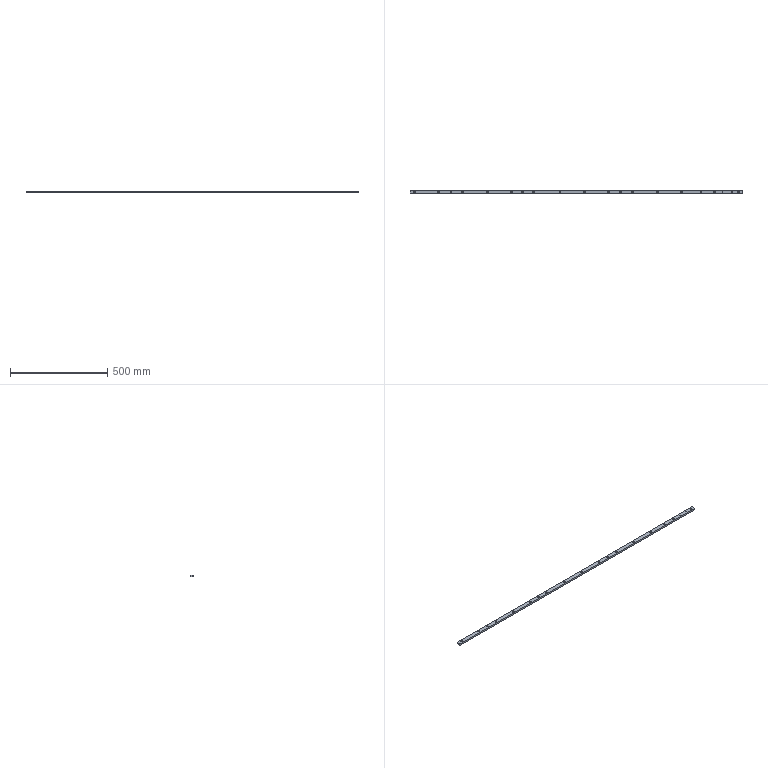Part | STEP file | J013-EBZ05-13-06-Part-1 | 1 solid | 62 faces | box 1710 x 19 x 9 mm | volume 279695 mm3 | cylinder 44 | plane 18 | commonest cylinder face diameters 10 x28 7 x12 5 x4